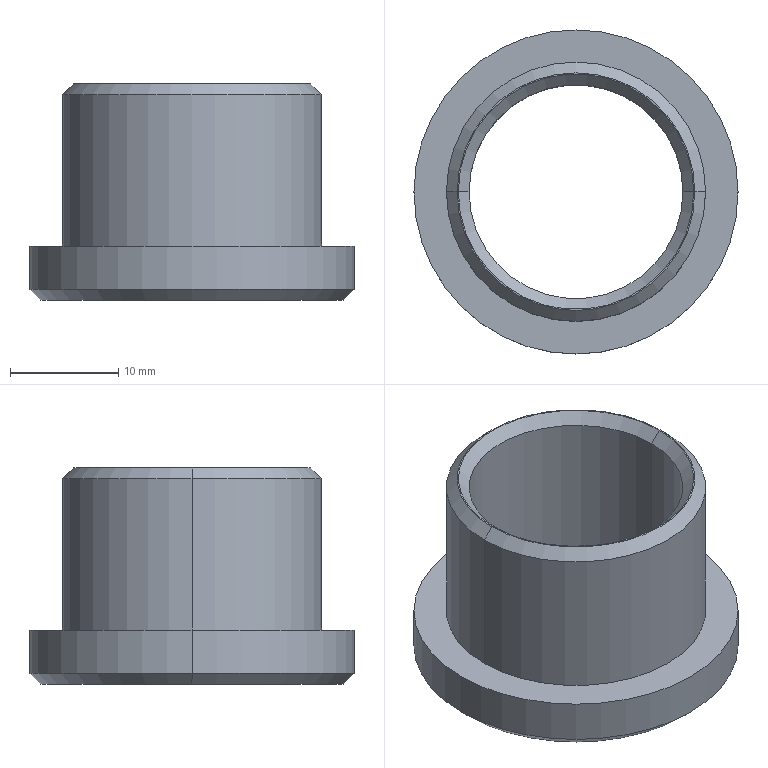Part | SolidWorks | features Chamfer 1, Extrusion 1, ICE 1 | 1 solid | 15 faces | box 30 x 30 x 20 mm | volume 4047 mm3 | cone 6 | cylinder 6 | plane 3 | commonest cylinder face diameters 19.8 x2 24 x2 30 x2
STEP:
#1=CARTESIAN_POINT('',(11.,0.,20.));
#2=VERTEX_POINT('',#1);
#3=CARTESIAN_POINT('',(-11.,0.,20.));
#4=VERTEX_POINT('',#3);
#5=CARTESIAN_POINT('',(0.,0.,20.));
#6=DIRECTION('',(0.,0.,1.));
#7=DIRECTION('',(1.,0.,0.));
#8=AXIS2_PLACEMENT_3D('',#5,#6,#7);
#9=CIRCLE('',#8,11.);
#10=EDGE_CURVE('',#2,#4,#9,.T.);
#11=ORIENTED_EDGE('',*,*,#10,.F.);
#12=CARTESIAN_POINT('',(12.,0.,19.));
#13=VERTEX_POINT('',#12);
#14=CARTESIAN_POINT('',(11.,0.,20.));
#15=DIRECTION('',(0.7071,0.,-0.7071));
#16=VECTOR('',#15,1000.);
#17=LINE('',#14,#16);
#18=EDGE_CURVE('',#2,#13,#17,.T.);
#19=ORIENTED_EDGE('',*,*,#18,.T.);
#20=CARTESIAN_POINT('',(-12.,0.,19.));
#21=VERTEX_POINT('',#20);
#22=CARTESIAN_POINT('',(0.,0.,19.));
#23=DIRECTION('',(0.,0.,-1.));
#24=DIRECTION('',(1.,0.,0.));
#25=AXIS2_PLACEMENT_3D('',#22,#23,#24);
#26=CIRCLE('',#25,12.);
#27=EDGE_CURVE('',#21,#13,#26,.T.);
#28=ORIENTED_EDGE('',*,*,#27,.F.);
#29=CARTESIAN_POINT('',(-11.,0.,20.));
#30=DIRECTION('',(-0.7071,0.,-0.7071));
#31=VECTOR('',#30,1000.);
#32=LINE('',#29,#31);
#33=EDGE_CURVE('',#4,#21,#32,.T.);
#34=ORIENTED_EDGE('',*,*,#33,.F.);
#35=EDGE_LOOP('',(#11,#19,#28,#34));
#36=FACE_OUTER_BOUND('',#35,.T.);
#37=CARTESIAN_POINT('',(0.,0.,20.));
#38=DIRECTION('',(0.,0.,-1.));
#39=DIRECTION('',(-1.,0.,0.));
#40=AXIS2_PLACEMENT_3D('',#37,#38,#39);
#41=CONICAL_SURFACE('',#40,11.,0.7854);
#42=ADVANCED_FACE('',(#36),#41,.T.);
#43=CARTESIAN_POINT('',(-14.,0.,0.));
#44=VERTEX_POINT('',#43);
#45=CARTESIAN_POINT('',(14.,0.,0.));
#46=VERTEX_POINT('',#45);
#47=CARTESIAN_POINT('',(0.,0.,0.));
#48=DIRECTION('',(0.,0.,-1.));
#49=DIRECTION('',(1.,0.,0.));
#50=AXIS2_PLACEMENT_3D('',#47,#48,#49);
#51=CIRCLE('',#50,14.);
#52=EDGE_CURVE('',#44,#46,#51,.T.);
#53=ORIENTED_EDGE('',*,*,#52,.F.);
#54=CARTESIAN_POINT('',(-15.,0.,1.));
#55=VERTEX_POINT('',#54);
#56=CARTESIAN_POINT('',(-15.,0.,1.));
#57=DIRECTION('',(-0.7071,0.,0.7071));
#58=VECTOR('',#57,1000.);
#59=LINE('',#56,#58);
#60=EDGE_CURVE('',#44,#55,#59,.T.);
#61=ORIENTED_EDGE('',*,*,#60,.T.);
#62=CARTESIAN_POINT('',(15.,0.,1.));
#63=VERTEX_POINT('',#62);
#64=CARTESIAN_POINT('',(0.,0.,1.));
#65=DIRECTION('',(0.,0.,1.));
#66=DIRECTION('',(1.,0.,0.));
#67=AXIS2_PLACEMENT_3D('',#64,#65,#66);
#68=CIRCLE('',#67,15.);
#69=EDGE_CURVE('',#63,#55,#68,.T.);
#70=ORIENTED_EDGE('',*,*,#69,.F.);
#71=CARTESIAN_POINT('',(15.,0.,1.));
#72=DIRECTION('',(0.7071,0.,0.7071));
#73=VECTOR('',#72,1000.);
#74=LINE('',#71,#73);
#75=EDGE_CURVE('',#46,#63,#74,.T.);
#76=ORIENTED_EDGE('',*,*,#75,.F.);
#77=EDGE_LOOP('',(#53,#61,#70,#76));
#78=FACE_OUTER_BOUND('',#77,.T.);
#79=CARTESIAN_POINT('',(0.,0.,1.));
#80=DIRECTION('',(0.,0.,1.));
#81=DIRECTION('',(1.,0.,0.));
#82=AXIS2_PLACEMENT_3D('',#79,#80,#81);
#83=CONICAL_SURFACE('',#82,15.,0.7854);
#84=ADVANCED_FACE('',(#78),#83,.T.);
#85=CARTESIAN_POINT('',(-9.9,0.,19.));
#86=VERTEX_POINT('',#85);
#87=CARTESIAN_POINT('',(9.9,0.,19.));
#88=VERTEX_POINT('',#87);
#89=CARTESIAN_POINT('',(0.,0.,19.));
#90=DIRECTION('',(0.,0.,1.));
#91=DIRECTION('',(1.,0.,0.));
#92=AXIS2_PLACEMENT_3D('',#89,#90,#91);
#93=CIRCLE('',#92,9.9);
#94=EDGE_CURVE('',#86,#88,#93,.T.);
#95=ORIENTED_EDGE('',*,*,#94,.F.);
#96=CARTESIAN_POINT('',(-10.9,0.,20.));
#97=VERTEX_POINT('',#96);
#98=CARTESIAN_POINT('',(-9.9,0.,19.));
#99=DIRECTION('',(-0.7071,0.,0.7071));
#100=VECTOR('',#99,1000.);
#101=LINE('',#98,#100);
#102=EDGE_CURVE('',#86,#97,#101,.T.);
#103=ORIENTED_EDGE('',*,*,#102,.T.);
#104=CARTESIAN_POINT('',(10.9,0.,20.));
#105=VERTEX_POINT('',#104);
#106=CARTESIAN_POINT('',(0.,0.,20.));
#107=DIRECTION('',(0.,0.,-1.));
#108=DIRECTION('',(1.,0.,0.));
#109=AXIS2_PLACEMENT_3D('',#106,#107,#108);
#110=CIRCLE('',#109,10.9);
#111=EDGE_CURVE('',#105,#97,#110,.T.);
#112=ORIENTED_EDGE('',*,*,#111,.F.);
#113=CARTESIAN_POINT('',(9.9,0.,19.));
#114=DIRECTION('',(0.7071,0.,0.7071));
#115=VECTOR('',#114,1000.);
#116=LINE('',#113,#115);
#117=EDGE_CURVE('',#88,#105,#116,.T.);
#118=ORIENTED_EDGE('',*,*,#117,.F.);
#119=EDGE_LOOP('',(#95,#103,#112,#118));
#120=FACE_OUTER_BOUND('',#119,.T.);
#121=CARTESIAN_POINT('',(0.,0.,19.));
#122=DIRECTION('',(0.,0.,1.));
#123=DIRECTION('',(1.,0.,0.));
#124=AXIS2_PLACEMENT_3D('',#121,#122,#123);
#125=CONICAL_SURFACE('',#124,9.9,0.7854);
#126=ADVANCED_FACE('',(#120),#125,.F.);
#127=ORIENTED_EDGE('',*,*,#27,.T.);
#128=CARTESIAN_POINT('',(12.,0.,5.));
#129=VERTEX_POINT('',#128);
#130=CARTESIAN_POINT('',(12.,0.,20.));
#131=DIRECTION('',(0.,0.,-1.));
#132=VECTOR('',#131,1000.);
#133=LINE('',#130,#132);
#134=EDGE_CURVE('',#13,#129,#133,.T.);
#135=ORIENTED_EDGE('',*,*,#134,.T.);
#136=CARTESIAN_POINT('',(-12.,0.,5.));
#137=VERTEX_POINT('',#136);
#138=CARTESIAN_POINT('',(0.,0.,5.));
#139=DIRECTION('',(0.,0.,1.));
#140=DIRECTION('',(1.,0.,0.));
#141=AXIS2_PLACEMENT_3D('',#138,#139,#140);
#142=CIRCLE('',#141,12.);
#143=EDGE_CURVE('',#129,#137,#142,.T.);
#144=ORIENTED_EDGE('',*,*,#143,.T.);
#145=CARTESIAN_POINT('',(-12.,0.,20.));
#146=DIRECTION('',(0.,0.,-1.));
#147=VECTOR('',#146,1000.);
#148=LINE('',#145,#147);
#149=EDGE_CURVE('',#21,#137,#148,.T.);
#150=ORIENTED_EDGE('',*,*,#149,.F.);
#151=EDGE_LOOP('',(#127,#135,#144,#150));
#152=FACE_OUTER_BOUND('',#151,.T.);
#153=CARTESIAN_POINT('',(0.,0.,20.));
#154=DIRECTION('',(0.,0.,-1.));
#155=DIRECTION('',(-1.,0.,0.));
#156=AXIS2_PLACEMENT_3D('',#153,#154,#155);
#157=CYLINDRICAL_SURFACE('',#156,12.);
#158=ADVANCED_FACE('',(#152),#157,.T.);
#159=ORIENTED_EDGE('',*,*,#94,.T.);
#160=CARTESIAN_POINT('',(9.9,0.,0.));
#161=VERTEX_POINT('',#160);
#162=CARTESIAN_POINT('',(9.9,0.,5.));
#163=DIRECTION('',(0.,0.,-1.));
#164=VECTOR('',#163,1000.);
#165=LINE('',#162,#164);
#166=EDGE_CURVE('',#88,#161,#165,.T.);
#167=ORIENTED_EDGE('',*,*,#166,.T.);
#168=CARTESIAN_POINT('',(-9.9,0.,0.));
#169=VERTEX_POINT('',#168);
#170=CARTESIAN_POINT('',(0.,0.,0.));
#171=DIRECTION('',(0.,0.,1.));
#172=DIRECTION('',(1.,0.,0.));
#173=AXIS2_PLACEMENT_3D('',#170,#171,#172);
#174=CIRCLE('',#173,9.9);
#175=EDGE_CURVE('',#169,#161,#174,.T.);
#176=ORIENTED_EDGE('',*,*,#175,.F.);
#177=CARTESIAN_POINT('',(-9.9,0.,5.));
#178=DIRECTION('',(0.,0.,-1.));
#179=VECTOR('',#178,1000.);
#180=LINE('',#177,#179);
#181=EDGE_CURVE('',#86,#169,#180,.T.);
#182=ORIENTED_EDGE('',*,*,#181,.F.);
#183=EDGE_LOOP('',(#159,#167,#176,#182));
#184=FACE_OUTER_BOUND('',#183,.T.);
#185=CARTESIAN_POINT('',(0.,0.,5.));
#186=DIRECTION('',(0.,0.,-1.));
#187=DIRECTION('',(-1.,0.,0.));
#188=AXIS2_PLACEMENT_3D('',#185,#186,#187);
#189=CYLINDRICAL_SURFACE('',#188,9.9);
#190=ADVANCED_FACE('',(#184),#189,.F.);
#191=CARTESIAN_POINT('',(15.,0.,5.));
#192=VERTEX_POINT('',#191);
#193=CARTESIAN_POINT('',(-15.,0.,5.));
#194=VERTEX_POINT('',#193);
#195=CARTESIAN_POINT('',(0.,0.,5.));
#196=DIRECTION('',(0.,0.,1.));
#197=DIRECTION('',(1.,0.,0.));
#198=AXIS2_PLACEMENT_3D('',#195,#196,#197);
#199=CIRCLE('',#198,15.);
#200=EDGE_CURVE('',#192,#194,#199,.T.);
#201=ORIENTED_EDGE('',*,*,#200,.F.);
#202=CARTESIAN_POINT('',(15.,0.,5.));
#203=DIRECTION('',(0.,0.,-1.));
#204=VECTOR('',#203,1000.);
#205=LINE('',#202,#204);
#206=EDGE_CURVE('',#192,#63,#205,.T.);
#207=ORIENTED_EDGE('',*,*,#206,.T.);
#208=ORIENTED_EDGE('',*,*,#69,.T.);
#209=CARTESIAN_POINT('',(-15.,0.,5.));
#210=DIRECTION('',(0.,0.,-1.));
#211=VECTOR('',#210,1000.);
#212=LINE('',#209,#211);
#213=EDGE_CURVE('',#194,#55,#212,.T.);
#214=ORIENTED_EDGE('',*,*,#213,.F.);
#215=EDGE_LOOP('',(#201,#207,#208,#214));
#216=FACE_OUTER_BOUND('',#215,.T.);
#217=CARTESIAN_POINT('',(0.,0.,5.));
#218=DIRECTION('',(0.,0.,-1.));
#219=DIRECTION('',(-1.,0.,0.));
#220=AXIS2_PLACEMENT_3D('',#217,#218,#219);
#221=CYLINDRICAL_SURFACE('',#220,15.);
#222=ADVANCED_FACE('',(#216),#221,.T.);
#223=CARTESIAN_POINT('',(0.,0.,5.));
#224=DIRECTION('',(0.,0.,1.));
#225=DIRECTION('',(1.,0.,0.));
#226=AXIS2_PLACEMENT_3D('',#223,#224,#225);
#227=CIRCLE('',#226,15.);
#228=EDGE_CURVE('',#194,#192,#227,.T.);
#229=ORIENTED_EDGE('',*,*,#228,.T.);
#230=ORIENTED_EDGE('',*,*,#200,.T.);
#231=EDGE_LOOP('',(#229,#230));
#232=FACE_OUTER_BOUND('',#231,.T.);
#233=CARTESIAN_POINT('',(0.,0.,5.));
#234=DIRECTION('',(0.,0.,1.));
#235=DIRECTION('',(1.,0.,0.));
#236=AXIS2_PLACEMENT_3D('',#233,#234,#235);
#237=CIRCLE('',#236,12.);
#238=EDGE_CURVE('',#137,#129,#237,.T.);
#239=ORIENTED_EDGE('',*,*,#238,.F.);
#240=ORIENTED_EDGE('',*,*,#143,.F.);
#241=EDGE_LOOP('',(#239,#240));
#242=FACE_BOUND('',#241,.T.);
#243=CARTESIAN_POINT('',(0.,0.,5.));
#244=DIRECTION('',(0.,0.,1.));
#245=DIRECTION('',(1.,0.,0.));
#246=AXIS2_PLACEMENT_3D('',#243,#244,#245);
#247=PLANE('',#246);
#248=ADVANCED_FACE('',(#232,#242),#247,.T.);
#249=CARTESIAN_POINT('',(0.,0.,0.));
#250=DIRECTION('',(0.,0.,-1.));
#251=DIRECTION('',(1.,0.,0.));
#252=AXIS2_PLACEMENT_3D('',#249,#250,#251);
#253=CIRCLE('',#252,14.);
#254=EDGE_CURVE('',#46,#44,#253,.T.);
#255=ORIENTED_EDGE('',*,*,#254,.T.);
#256=ORIENTED_EDGE('',*,*,#52,.T.);
#257=EDGE_LOOP('',(#255,#256));
#258=FACE_OUTER_BOUND('',#257,.T.);
#259=ORIENTED_EDGE('',*,*,#175,.T.);
#260=CARTESIAN_POINT('',(0.,0.,0.));
#261=DIRECTION('',(0.,0.,1.));
#262=DIRECTION('',(1.,0.,0.));
#263=AXIS2_PLACEMENT_3D('',#260,#261,#262);
#264=CIRCLE('',#263,9.9);
#265=EDGE_CURVE('',#161,#169,#264,.T.);
#266=ORIENTED_EDGE('',*,*,#265,.T.);
#267=EDGE_LOOP('',(#259,#266));
#268=FACE_BOUND('',#267,.T.);
#269=CARTESIAN_POINT('',(0.,0.,0.));
#270=DIRECTION('',(0.,0.,1.));
#271=DIRECTION('',(1.,0.,0.));
#272=AXIS2_PLACEMENT_3D('',#269,#270,#271);
#273=PLANE('',#272);
#274=ADVANCED_FACE('',(#258,#268),#273,.F.);
#275=ORIENTED_EDGE('',*,*,#206,.F.);
#276=ORIENTED_EDGE('',*,*,#228,.F.);
#277=ORIENTED_EDGE('',*,*,#213,.T.);
#278=CARTESIAN_POINT('',(0.,0.,1.));
#279=DIRECTION('',(0.,0.,1.));
#280=DIRECTION('',(1.,0.,0.));
#281=AXIS2_PLACEMENT_3D('',#278,#279,#280);
#282=CIRCLE('',#281,15.);
#283=EDGE_CURVE('',#55,#63,#282,.T.);
#284=ORIENTED_EDGE('',*,*,#283,.T.);
#285=EDGE_LOOP('',(#275,#276,#277,#284));
#286=FACE_OUTER_BOUND('',#285,.T.);
#287=CARTESIAN_POINT('',(0.,0.,5.));
#288=DIRECTION('',(0.,0.,-1.));
#289=DIRECTION('',(-1.,0.,0.));
#290=AXIS2_PLACEMENT_3D('',#287,#288,#289);
#291=CYLINDRICAL_SURFACE('',#290,15.);
#292=ADVANCED_FACE('',(#286),#291,.T.);
#293=ORIENTED_EDGE('',*,*,#166,.F.);
#294=CARTESIAN_POINT('',(0.,0.,19.));
#295=DIRECTION('',(0.,0.,1.));
#296=DIRECTION('',(1.,0.,0.));
#297=AXIS2_PLACEMENT_3D('',#294,#295,#296);
#298=CIRCLE('',#297,9.9);
#299=EDGE_CURVE('',#88,#86,#298,.T.);
#300=ORIENTED_EDGE('',*,*,#299,.T.);
#301=ORIENTED_EDGE('',*,*,#181,.T.);
#302=ORIENTED_EDGE('',*,*,#265,.F.);
#303=EDGE_LOOP('',(#293,#300,#301,#302));
#304=FACE_OUTER_BOUND('',#303,.T.);
#305=CARTESIAN_POINT('',(0.,0.,5.));
#306=DIRECTION('',(0.,0.,-1.));
#307=DIRECTION('',(-1.,0.,0.));
#308=AXIS2_PLACEMENT_3D('',#305,#306,#307);
#309=CYLINDRICAL_SURFACE('',#308,9.9);
#310=ADVANCED_FACE('',(#304),#309,.F.);
#311=ORIENTED_EDGE('',*,*,#111,.T.);
#312=CARTESIAN_POINT('',(0.,0.,20.));
#313=DIRECTION('',(0.,0.,-1.));
#314=DIRECTION('',(1.,0.,0.));
#315=AXIS2_PLACEMENT_3D('',#312,#313,#314);
#316=CIRCLE('',#315,10.9);
#317=EDGE_CURVE('',#97,#105,#316,.T.);
#318=ORIENTED_EDGE('',*,*,#317,.T.);
#319=EDGE_LOOP('',(#311,#318));
#320=FACE_BOUND('',#319,.T.);
#321=CARTESIAN_POINT('',(0.,0.,20.));
#322=DIRECTION('',(0.,0.,1.));
#323=DIRECTION('',(1.,0.,0.));
#324=AXIS2_PLACEMENT_3D('',#321,#322,#323);
#325=CIRCLE('',#324,11.);
#326=EDGE_CURVE('',#4,#2,#325,.T.);
#327=ORIENTED_EDGE('',*,*,#326,.T.);
#328=ORIENTED_EDGE('',*,*,#10,.T.);
#329=EDGE_LOOP('',(#327,#328));
#330=FACE_OUTER_BOUND('',#329,.T.);
#331=CARTESIAN_POINT('',(0.,0.,20.));
#332=DIRECTION('',(0.,0.,1.));
#333=DIRECTION('',(1.,0.,0.));
#334=AXIS2_PLACEMENT_3D('',#331,#332,#333);
#335=PLANE('',#334);
#336=ADVANCED_FACE('',(#320,#330),#335,.T.);
#337=ORIENTED_EDGE('',*,*,#134,.F.);
#338=CARTESIAN_POINT('',(0.,0.,19.));
#339=DIRECTION('',(0.,0.,-1.));
#340=DIRECTION('',(1.,0.,0.));
#341=AXIS2_PLACEMENT_3D('',#338,#339,#340);
#342=CIRCLE('',#341,12.);
#343=EDGE_CURVE('',#13,#21,#342,.T.);
#344=ORIENTED_EDGE('',*,*,#343,.T.);
#345=ORIENTED_EDGE('',*,*,#149,.T.);
#346=ORIENTED_EDGE('',*,*,#238,.T.);
#347=EDGE_LOOP('',(#337,#344,#345,#346));
#348=FACE_OUTER_BOUND('',#347,.T.);
#349=CARTESIAN_POINT('',(0.,0.,20.));
#350=DIRECTION('',(0.,0.,-1.));
#351=DIRECTION('',(-1.,0.,0.));
#352=AXIS2_PLACEMENT_3D('',#349,#350,#351);
#353=CYLINDRICAL_SURFACE('',#352,12.);
#354=ADVANCED_FACE('',(#348),#353,.T.);
#355=ORIENTED_EDGE('',*,*,#102,.F.);
#356=ORIENTED_EDGE('',*,*,#299,.F.);
#357=ORIENTED_EDGE('',*,*,#117,.T.);
#358=ORIENTED_EDGE('',*,*,#317,.F.);
#359=EDGE_LOOP('',(#355,#356,#357,#358));
#360=FACE_OUTER_BOUND('',#359,.T.);
#361=CARTESIAN_POINT('',(0.,0.,19.));
#362=DIRECTION('',(0.,0.,1.));
#363=DIRECTION('',(1.,0.,0.));
#364=AXIS2_PLACEMENT_3D('',#361,#362,#363);
#365=CONICAL_SURFACE('',#364,9.9,0.7854);
#366=ADVANCED_FACE('',(#360),#365,.F.);
#367=ORIENTED_EDGE('',*,*,#60,.F.);
#368=ORIENTED_EDGE('',*,*,#254,.F.);
#369=ORIENTED_EDGE('',*,*,#75,.T.);
#370=ORIENTED_EDGE('',*,*,#283,.F.);
#371=EDGE_LOOP('',(#367,#368,#369,#370));
#372=FACE_OUTER_BOUND('',#371,.T.);
#373=CARTESIAN_POINT('',(0.,0.,1.));
#374=DIRECTION('',(0.,0.,1.));
#375=DIRECTION('',(1.,0.,0.));
#376=AXIS2_PLACEMENT_3D('',#373,#374,#375);
#377=CONICAL_SURFACE('',#376,15.,0.7854);
#378=ADVANCED_FACE('',(#372),#377,.T.);
#379=ORIENTED_EDGE('',*,*,#18,.F.);
#380=ORIENTED_EDGE('',*,*,#326,.F.);
#381=ORIENTED_EDGE('',*,*,#33,.T.);
#382=ORIENTED_EDGE('',*,*,#343,.F.);
#383=EDGE_LOOP('',(#379,#380,#381,#382));
#384=FACE_OUTER_BOUND('',#383,.T.);
#385=CARTESIAN_POINT('',(0.,0.,20.));
#386=DIRECTION('',(0.,0.,-1.));
#387=DIRECTION('',(-1.,0.,0.));
#388=AXIS2_PLACEMENT_3D('',#385,#386,#387);
#389=CONICAL_SURFACE('',#388,11.,0.7854);
#390=ADVANCED_FACE('',(#384),#389,.T.);
#391=CLOSED_SHELL('',(#42,#84,#126,#158,#190,#222,#248,#274,#292,#310,#336,#354,#366,#378,#390));
#392=MANIFOLD_SOLID_BREP('',#391);
#393=CARTESIAN_POINT('',(0.,0.,0.));
#394=DIRECTION('',(0.,0.,1.));
#395=DIRECTION('',(1.,0.,0.));
#396=AXIS2_PLACEMENT_3D('',#393,#394,#395);
#397=(LENGTH_UNIT()NAMED_UNIT(*)SI_UNIT(.MILLI.,.METRE.));
#398=UNCERTAINTY_MEASURE_WITH_UNIT(LENGTH_MEASURE(0.00001),#397,'','');
#399=(NAMED_UNIT(*)PLANE_ANGLE_UNIT()SI_UNIT($,.RADIAN.));
#400=(NAMED_UNIT(*)SI_UNIT($,.STERADIAN.)SOLID_ANGLE_UNIT());
#401=(GEOMETRIC_REPRESENTATION_CONTEXT(3)GLOBAL_UNCERTAINTY_ASSIGNED_CONTEXT((#398))GLOBAL_UNIT_ASSIGNED_CONTEXT((#397,#399,#400))REPRESENTATION_CONTEXT('',''));
#402=ADVANCED_BREP_SHAPE_REPRESENTATION('',(#392,#396),#401);